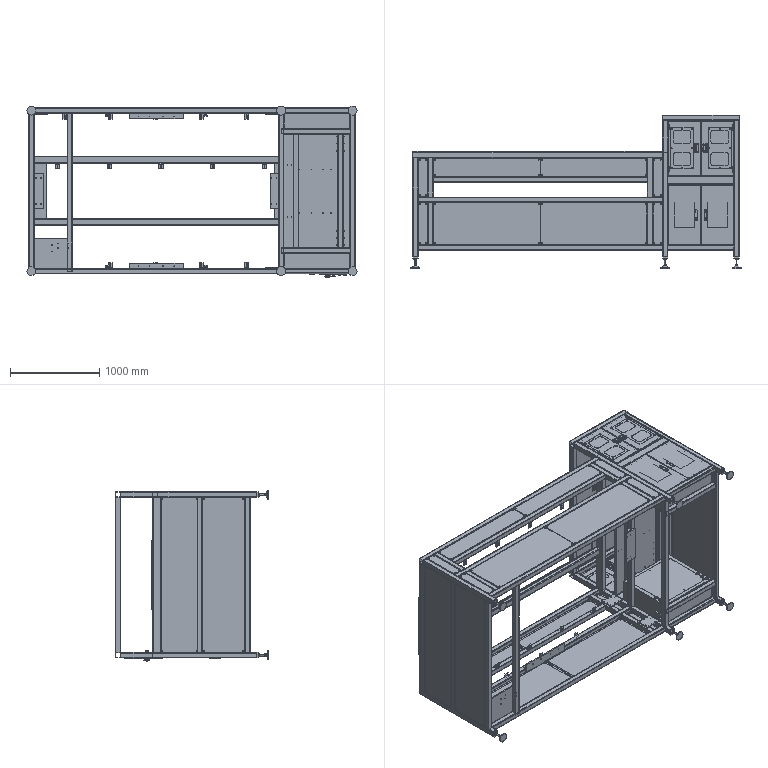Part | SolidWorks | features CompositeCurve 5, ReferencePattern 4, LocalLPattern 3 | 246 solids | 7273 faces | volume 137447559 mm3 | plane 4225 | cylinder 2673 | spline 206 | cone 87 | torus 82 | commonest cylinder face diameters 5 x456 7 x173 6.6 x164 11 x164 6.4 x140 12.8 x140